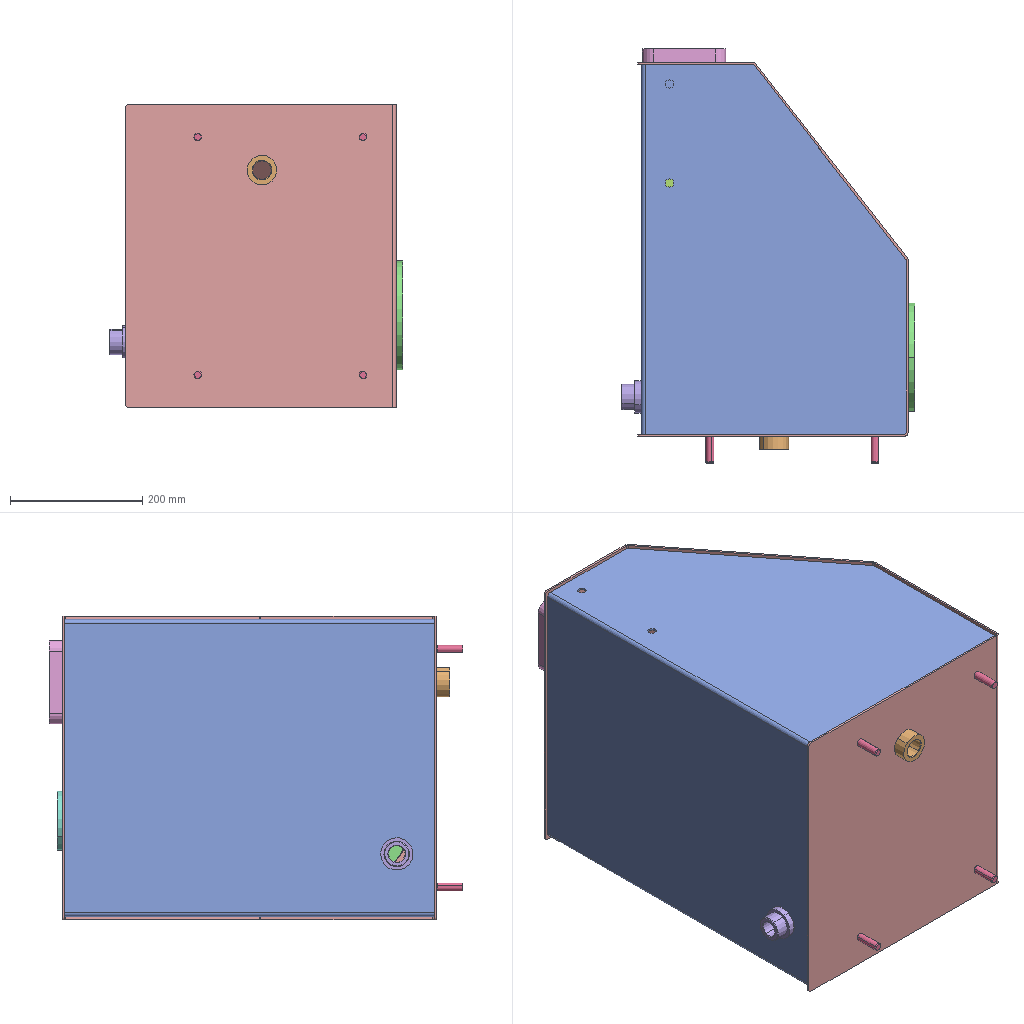Assembly | SolidWorks | 9 different items | 12 placed | box 444 x 626 x 460 mm
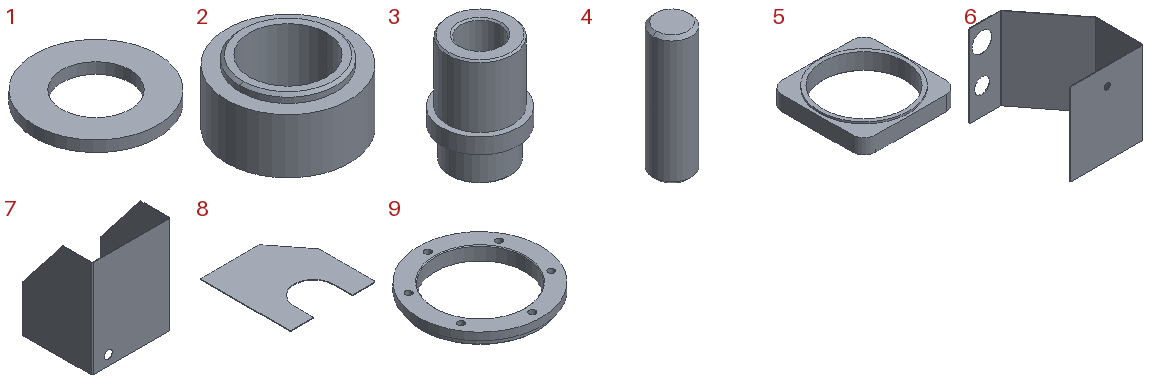Parts list (item | quantity | size | volume | features):
1 | x1 | 90 x 90 x 8 mm | 34479 mm3 | features ICE 2, Chamfer 1, Cut 1, Extrusion 1
2 | x1 | 45 x 45 x 23 mm | 20434 mm3 | features Chamfer 1, Extrusion 1, ICE 1
3 | x1 | 48.99 x 48.99 x 70 mm | 63043 mm3 | features ICE 2, Chamfer 1, Extrusion 1
4 | x4 | 11.85 x 11.85 x 40 mm | 4376 mm3 | features Chamfer 1, Extrusion 1
5 | x1 | 126 x 126 x 22.5 mm | 124484 mm3 | features 3DProfileFeature 1, Chamfer 1, Extrusion 1, HoleWzd 1, ICE 1
6 | x1 | 409 x 566 x 460 mm | 1582999 mm3 | features Cut 3, FlatPattern 1, ICE 1, SMBaseFlange 1, SheetMetal 1
7 | x1 | 450 x 401 x 560 mm | 1875203 mm3 | features ICE 2, Cut 1, FlatPattern 1, SMBaseFlange 1, SheetMetal 1
8 | x1 | 398 x 420 x 3 mm | 386101 mm3 | features Extrusion 1
9 | x1 | 165 x 165 x 18 mm | 159935 mm3 | features ICE 2, Chamfer 1, Extrusion 1
Mates (type | each side: item.copy, entity, surface, feature):
Coincident | 6.1 face plane Base-Flange1 | 7.1 face plane Base-Flange1 | 2 times
DistanceDim | 7.1 face plane Base-Flange1 | 6.1 face plane Base-Flange1
Coincident | 6.1 face plane Base-Flange1 | 8.1 face plane Boss-Extrude1 | 2 times
DistanceDim | 8.1 face plane Boss-Extrude1 | 6.1 face plane Base-Bend3
Coincident | 6.1 face plane Base-Flange1 | 5.1 face plane Boss-Extrude1
Parallel | 7.1 face plane Base-Flange1 | 5.1 face plane Boss-Extrude1
Coincident | 6.1 face plane Base-Flange1 | 1.1 face plane Boss-Extrude1
Coincident | 7.1 face plane Base-Flange1 | 3.1 face plane Boss-Extrude2
Concentric | 7.1 edge | 3.1 edge
Coincident | 6.1 face plane Base-Flange1 | 2.1 face plane Boss-Extrude1
Concentric | 6.1 edge | 1.1 edge
Concentric | 6.1 edge | 5.1 edge
Concentric | 6.1 edge | 2.1 edge
Concentric | 6.1 edge | 9.1 edge
Coincident | 6.1 face plane Base-Flange1 | 9.1 face plane Boss-Extrude1
Coincident | 6.1 face plane Base-Flange1 | 4.1 face plane Boss-Extrude1
Coincident | 6.1 face plane Base-Flange1 | 4.2 face plane Boss-Extrude1
Coincident | 6.1 face plane Base-Flange1 | 4.3 face plane Boss-Extrude1
Coincident | 6.1 face plane Base-Flange1 | 4.4 face plane Boss-Extrude1
Concentric | 4.2 edge | assembly select_type:10
Concentric | 4.4 edge | assembly select_type:10
Concentric | 4.1 edge | assembly select_type:10
Concentric | 4.3 edge | assembly select_type:10